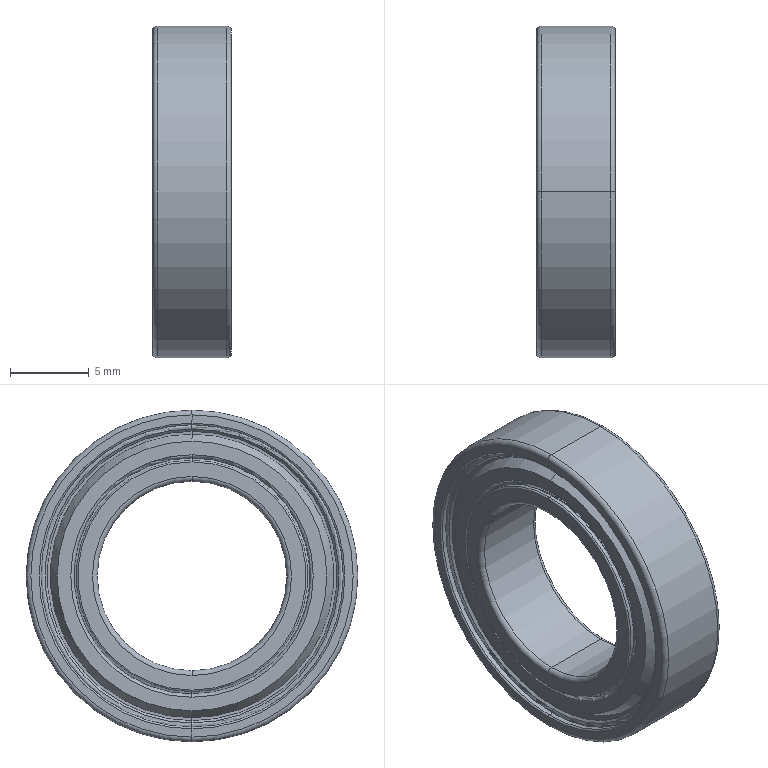Part | NX | features BREP 1 | 1 solid | 139 faces | box 5 x 21 x 21 mm | volume 897.771 mm3 | torus 54 | cone 50 | cylinder 24 | plane 11 | commonest cylinder face diameters 14.65 x4 14.95 x4 15.25 x4 15.35 x4 19.15 x4 12 x2